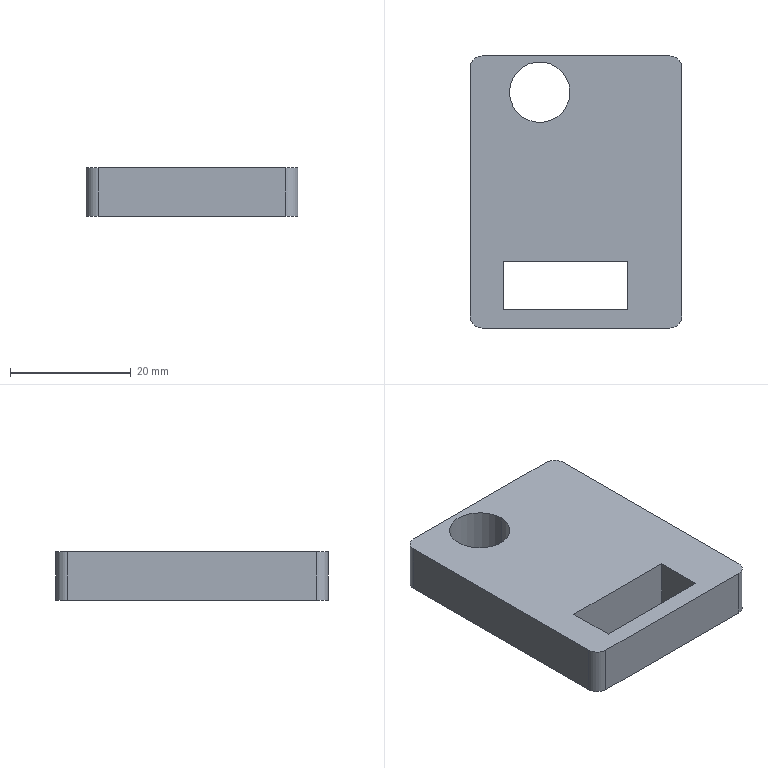Part | SolidWorks | features Fillet 1, FlatPattern 1, SMBaseFlange 1, SheetMetal 1 | 1 solid | 16 faces | box 35 x 45 x 8 mm | volume 10632 mm3 | plane 10 | cylinder 6 | commonest cylinder face diameters 4 x4 10 x2
STEP:
#1=CARTESIAN_POINT('',(-109.081,0.,8.));
#2=VERTEX_POINT('',#1);
#3=CARTESIAN_POINT('',(-99.081,0.,8.));
#4=VERTEX_POINT('',#3);
#5=CARTESIAN_POINT('',(-104.081,0.,8.));
#6=DIRECTION('',(0.,0.,1.));
#7=DIRECTION('',(1.,0.,0.));
#8=AXIS2_PLACEMENT_3D('',#5,#6,#7);
#9=CIRCLE('',#8,5.);
#10=EDGE_CURVE('',#2,#4,#9,.T.);
#11=ORIENTED_EDGE('',*,*,#10,.T.);
#12=CARTESIAN_POINT('',(-99.081,0.,0.));
#13=VERTEX_POINT('',#12);
#14=CARTESIAN_POINT('',(-99.081,0.,8.));
#15=DIRECTION('',(0.,0.,-1.));
#16=VECTOR('',#15,1000.);
#17=LINE('',#14,#16);
#18=EDGE_CURVE('',#4,#13,#17,.T.);
#19=ORIENTED_EDGE('',*,*,#18,.T.);
#20=CARTESIAN_POINT('',(-109.081,0.,0.));
#21=VERTEX_POINT('',#20);
#22=CARTESIAN_POINT('',(-104.081,0.,0.));
#23=DIRECTION('',(0.,0.,1.));
#24=DIRECTION('',(1.,0.,0.));
#25=AXIS2_PLACEMENT_3D('',#22,#23,#24);
#26=CIRCLE('',#25,5.);
#27=EDGE_CURVE('',#21,#13,#26,.T.);
#28=ORIENTED_EDGE('',*,*,#27,.F.);
#29=CARTESIAN_POINT('',(-109.081,0.,8.));
#30=DIRECTION('',(0.,0.,-1.));
#31=VECTOR('',#30,1000.);
#32=LINE('',#29,#31);
#33=EDGE_CURVE('',#2,#21,#32,.T.);
#34=ORIENTED_EDGE('',*,*,#33,.F.);
#35=EDGE_LOOP('',(#11,#19,#28,#34));
#36=FACE_OUTER_BOUND('',#35,.T.);
#37=CARTESIAN_POINT('',(-104.081,0.,8.));
#38=DIRECTION('',(0.,0.,-1.));
#39=DIRECTION('',(-1.,0.,0.));
#40=AXIS2_PLACEMENT_3D('',#37,#38,#39);
#41=CYLINDRICAL_SURFACE('',#40,5.);
#42=ADVANCED_FACE('',(#36),#41,.F.);
#43=ORIENTED_EDGE('',*,*,#10,.F.);
#44=CARTESIAN_POINT('',(-104.081,0.,8.));
#45=DIRECTION('',(0.,0.,1.));
#46=DIRECTION('',(1.,0.,0.));
#47=AXIS2_PLACEMENT_3D('',#44,#45,#46);
#48=CIRCLE('',#47,5.);
#49=EDGE_CURVE('',#4,#2,#48,.T.);
#50=ORIENTED_EDGE('',*,*,#49,.F.);
#51=EDGE_LOOP('',(#43,#50));
#52=FACE_BOUND('',#51,.T.);
#53=CARTESIAN_POINT('',(-115.581,4.,8.));
#54=VERTEX_POINT('',#53);
#55=CARTESIAN_POINT('',(-115.581,-37.,8.));
#56=VERTEX_POINT('',#55);
#57=CARTESIAN_POINT('',(-115.581,-39.,8.));
#58=DIRECTION('',(0.,-1.,0.));
#59=VECTOR('',#58,1000.);
#60=LINE('',#57,#59);
#61=EDGE_CURVE('',#54,#56,#60,.T.);
#62=ORIENTED_EDGE('',*,*,#61,.T.);
#63=CARTESIAN_POINT('',(-113.581,-39.,8.));
#64=VERTEX_POINT('',#63);
#65=CARTESIAN_POINT('',(-113.581,-37.,8.));
#66=DIRECTION('',(0.,0.,1.));
#67=DIRECTION('',(-1.,0.,0.));
#68=AXIS2_PLACEMENT_3D('',#65,#66,#67);
#69=CIRCLE('',#68,2.);
#70=EDGE_CURVE('',#56,#64,#69,.T.);
#71=ORIENTED_EDGE('',*,*,#70,.T.);
#72=CARTESIAN_POINT('',(-82.581,-39.,8.));
#73=VERTEX_POINT('',#72);
#74=CARTESIAN_POINT('',(-80.581,-39.,8.));
#75=DIRECTION('',(1.,0.,0.));
#76=VECTOR('',#75,1000.);
#77=LINE('',#74,#76);
#78=EDGE_CURVE('',#64,#73,#77,.T.);
#79=ORIENTED_EDGE('',*,*,#78,.T.);
#80=CARTESIAN_POINT('',(-80.581,-37.,8.));
#81=VERTEX_POINT('',#80);
#82=CARTESIAN_POINT('',(-82.581,-37.,8.));
#83=DIRECTION('',(0.,0.,1.));
#84=DIRECTION('',(-1.,0.,0.));
#85=AXIS2_PLACEMENT_3D('',#82,#83,#84);
#86=CIRCLE('',#85,2.);
#87=EDGE_CURVE('',#73,#81,#86,.T.);
#88=ORIENTED_EDGE('',*,*,#87,.T.);
#89=CARTESIAN_POINT('',(-80.581,4.,8.));
#90=VERTEX_POINT('',#89);
#91=CARTESIAN_POINT('',(-80.581,6.,8.));
#92=DIRECTION('',(0.,1.,0.));
#93=VECTOR('',#92,1000.);
#94=LINE('',#91,#93);
#95=EDGE_CURVE('',#81,#90,#94,.T.);
#96=ORIENTED_EDGE('',*,*,#95,.T.);
#97=CARTESIAN_POINT('',(-82.581,6.,8.));
#98=VERTEX_POINT('',#97);
#99=CARTESIAN_POINT('',(-82.581,4.,8.));
#100=DIRECTION('',(0.,0.,1.));
#101=DIRECTION('',(-1.,0.,0.));
#102=AXIS2_PLACEMENT_3D('',#99,#100,#101);
#103=CIRCLE('',#102,2.);
#104=EDGE_CURVE('',#90,#98,#103,.T.);
#105=ORIENTED_EDGE('',*,*,#104,.T.);
#106=CARTESIAN_POINT('',(-113.581,6.,8.));
#107=VERTEX_POINT('',#106);
#108=CARTESIAN_POINT('',(-115.581,6.,8.));
#109=DIRECTION('',(-1.,0.,0.));
#110=VECTOR('',#109,1000.);
#111=LINE('',#108,#110);
#112=EDGE_CURVE('',#98,#107,#111,.T.);
#113=ORIENTED_EDGE('',*,*,#112,.T.);
#114=CARTESIAN_POINT('',(-113.581,4.,8.));
#115=DIRECTION('',(0.,0.,1.));
#116=DIRECTION('',(-1.,0.,0.));
#117=AXIS2_PLACEMENT_3D('',#114,#115,#116);
#118=CIRCLE('',#117,2.);
#119=EDGE_CURVE('',#107,#54,#118,.T.);
#120=ORIENTED_EDGE('',*,*,#119,.T.);
#121=EDGE_LOOP('',(#62,#71,#79,#88,#96,#105,#113,#120));
#122=FACE_OUTER_BOUND('',#121,.T.);
#123=CARTESIAN_POINT('',(-110.081,-28.,8.));
#124=VERTEX_POINT('',#123);
#125=CARTESIAN_POINT('',(-110.081,-36.,8.));
#126=VERTEX_POINT('',#125);
#127=CARTESIAN_POINT('',(-110.081,-36.,8.));
#128=DIRECTION('',(0.,-1.,0.));
#129=VECTOR('',#128,1000.);
#130=LINE('',#127,#129);
#131=EDGE_CURVE('',#124,#126,#130,.T.);
#132=ORIENTED_EDGE('',*,*,#131,.F.);
#133=CARTESIAN_POINT('',(-89.581,-28.,8.));
#134=VERTEX_POINT('',#133);
#135=CARTESIAN_POINT('',(-110.081,-28.,8.));
#136=DIRECTION('',(-1.,0.,0.));
#137=VECTOR('',#136,1000.);
#138=LINE('',#135,#137);
#139=EDGE_CURVE('',#134,#124,#138,.T.);
#140=ORIENTED_EDGE('',*,*,#139,.F.);
#141=CARTESIAN_POINT('',(-89.581,-36.,8.));
#142=VERTEX_POINT('',#141);
#143=CARTESIAN_POINT('',(-89.581,-28.,8.));
#144=DIRECTION('',(0.,1.,0.));
#145=VECTOR('',#144,1000.);
#146=LINE('',#143,#145);
#147=EDGE_CURVE('',#142,#134,#146,.T.);
#148=ORIENTED_EDGE('',*,*,#147,.F.);
#149=CARTESIAN_POINT('',(-89.581,-36.,8.));
#150=DIRECTION('',(1.,0.,0.));
#151=VECTOR('',#150,1000.);
#152=LINE('',#149,#151);
#153=EDGE_CURVE('',#126,#142,#152,.T.);
#154=ORIENTED_EDGE('',*,*,#153,.F.);
#155=EDGE_LOOP('',(#132,#140,#148,#154));
#156=FACE_BOUND('',#155,.T.);
#157=CARTESIAN_POINT('',(0.,0.,8.));
#158=DIRECTION('',(0.,0.,-1.));
#159=DIRECTION('',(-1.,0.,0.));
#160=AXIS2_PLACEMENT_3D('',#157,#158,#159);
#161=PLANE('',#160);
#162=ADVANCED_FACE('',(#52,#122,#156),#161,.F.);
#163=CARTESIAN_POINT('',(-113.581,-39.,0.));
#164=VERTEX_POINT('',#163);
#165=CARTESIAN_POINT('',(-82.581,-39.,0.));
#166=VERTEX_POINT('',#165);
#167=CARTESIAN_POINT('',(-80.581,-39.,0.));
#168=DIRECTION('',(1.,0.,0.));
#169=VECTOR('',#168,1000.);
#170=LINE('',#167,#169);
#171=EDGE_CURVE('',#164,#166,#170,.T.);
#172=ORIENTED_EDGE('',*,*,#171,.F.);
#173=CARTESIAN_POINT('',(-115.581,-37.,0.));
#174=VERTEX_POINT('',#173);
#175=CARTESIAN_POINT('',(-113.581,-37.,0.));
#176=DIRECTION('',(0.,0.,-1.));
#177=DIRECTION('',(-1.,0.,0.));
#178=AXIS2_PLACEMENT_3D('',#175,#176,#177);
#179=CIRCLE('',#178,2.);
#180=EDGE_CURVE('',#164,#174,#179,.T.);
#181=ORIENTED_EDGE('',*,*,#180,.T.);
#182=CARTESIAN_POINT('',(-115.581,4.,0.));
#183=VERTEX_POINT('',#182);
#184=CARTESIAN_POINT('',(-115.581,-39.,0.));
#185=DIRECTION('',(0.,-1.,0.));
#186=VECTOR('',#185,1000.);
#187=LINE('',#184,#186);
#188=EDGE_CURVE('',#183,#174,#187,.T.);
#189=ORIENTED_EDGE('',*,*,#188,.F.);
#190=CARTESIAN_POINT('',(-113.581,6.,0.));
#191=VERTEX_POINT('',#190);
#192=CARTESIAN_POINT('',(-113.581,4.,0.));
#193=DIRECTION('',(0.,0.,-1.));
#194=DIRECTION('',(-1.,0.,0.));
#195=AXIS2_PLACEMENT_3D('',#192,#193,#194);
#196=CIRCLE('',#195,2.);
#197=EDGE_CURVE('',#183,#191,#196,.T.);
#198=ORIENTED_EDGE('',*,*,#197,.T.);
#199=CARTESIAN_POINT('',(-82.581,6.,0.));
#200=VERTEX_POINT('',#199);
#201=CARTESIAN_POINT('',(-115.581,6.,0.));
#202=DIRECTION('',(-1.,0.,0.));
#203=VECTOR('',#202,1000.);
#204=LINE('',#201,#203);
#205=EDGE_CURVE('',#200,#191,#204,.T.);
#206=ORIENTED_EDGE('',*,*,#205,.F.);
#207=CARTESIAN_POINT('',(-80.581,4.,0.));
#208=VERTEX_POINT('',#207);
#209=CARTESIAN_POINT('',(-82.581,4.,0.));
#210=DIRECTION('',(0.,0.,-1.));
#211=DIRECTION('',(-1.,0.,0.));
#212=AXIS2_PLACEMENT_3D('',#209,#210,#211);
#213=CIRCLE('',#212,2.);
#214=EDGE_CURVE('',#200,#208,#213,.T.);
#215=ORIENTED_EDGE('',*,*,#214,.T.);
#216=CARTESIAN_POINT('',(-80.581,-37.,0.));
#217=VERTEX_POINT('',#216);
#218=CARTESIAN_POINT('',(-80.581,6.,0.));
#219=DIRECTION('',(0.,1.,0.));
#220=VECTOR('',#219,1000.);
#221=LINE('',#218,#220);
#222=EDGE_CURVE('',#217,#208,#221,.T.);
#223=ORIENTED_EDGE('',*,*,#222,.F.);
#224=CARTESIAN_POINT('',(-82.581,-37.,0.));
#225=DIRECTION('',(0.,0.,-1.));
#226=DIRECTION('',(-1.,0.,0.));
#227=AXIS2_PLACEMENT_3D('',#224,#225,#226);
#228=CIRCLE('',#227,2.);
#229=EDGE_CURVE('',#217,#166,#228,.T.);
#230=ORIENTED_EDGE('',*,*,#229,.T.);
#231=EDGE_LOOP('',(#172,#181,#189,#198,#206,#215,#223,#230));
#232=FACE_OUTER_BOUND('',#231,.T.);
#233=ORIENTED_EDGE('',*,*,#27,.T.);
#234=CARTESIAN_POINT('',(-104.081,0.,0.));
#235=DIRECTION('',(0.,0.,1.));
#236=DIRECTION('',(1.,0.,0.));
#237=AXIS2_PLACEMENT_3D('',#234,#235,#236);
#238=CIRCLE('',#237,5.);
#239=EDGE_CURVE('',#13,#21,#238,.T.);
#240=ORIENTED_EDGE('',*,*,#239,.T.);
#241=EDGE_LOOP('',(#233,#240));
#242=FACE_BOUND('',#241,.T.);
#243=CARTESIAN_POINT('',(-89.581,-28.,0.));
#244=VERTEX_POINT('',#243);
#245=CARTESIAN_POINT('',(-110.081,-28.,0.));
#246=VERTEX_POINT('',#245);
#247=CARTESIAN_POINT('',(-110.081,-28.,0.));
#248=DIRECTION('',(-1.,0.,0.));
#249=VECTOR('',#248,1000.);
#250=LINE('',#247,#249);
#251=EDGE_CURVE('',#244,#246,#250,.T.);
#252=ORIENTED_EDGE('',*,*,#251,.T.);
#253=CARTESIAN_POINT('',(-110.081,-36.,0.));
#254=VERTEX_POINT('',#253);
#255=CARTESIAN_POINT('',(-110.081,-36.,0.));
#256=DIRECTION('',(0.,-1.,0.));
#257=VECTOR('',#256,1000.);
#258=LINE('',#255,#257);
#259=EDGE_CURVE('',#246,#254,#258,.T.);
#260=ORIENTED_EDGE('',*,*,#259,.T.);
#261=CARTESIAN_POINT('',(-89.581,-36.,0.));
#262=VERTEX_POINT('',#261);
#263=CARTESIAN_POINT('',(-89.581,-36.,0.));
#264=DIRECTION('',(1.,0.,0.));
#265=VECTOR('',#264,1000.);
#266=LINE('',#263,#265);
#267=EDGE_CURVE('',#254,#262,#266,.T.);
#268=ORIENTED_EDGE('',*,*,#267,.T.);
#269=CARTESIAN_POINT('',(-89.581,-28.,0.));
#270=DIRECTION('',(0.,1.,0.));
#271=VECTOR('',#270,1000.);
#272=LINE('',#269,#271);
#273=EDGE_CURVE('',#262,#244,#272,.T.);
#274=ORIENTED_EDGE('',*,*,#273,.T.);
#275=EDGE_LOOP('',(#252,#260,#268,#274));
#276=FACE_BOUND('',#275,.T.);
#277=CARTESIAN_POINT('',(0.,0.,0.));
#278=DIRECTION('',(0.,0.,-1.));
#279=DIRECTION('',(-1.,0.,0.));
#280=AXIS2_PLACEMENT_3D('',#277,#278,#279);
#281=PLANE('',#280);
#282=ADVANCED_FACE('',(#232,#242,#276),#281,.T.);
#283=ORIENTED_EDGE('',*,*,#188,.T.);
#284=CARTESIAN_POINT('',(-115.581,-37.,8.));
#285=DIRECTION('',(0.,0.,1.));
#286=VECTOR('',#285,1000.);
#287=LINE('',#284,#286);
#288=EDGE_CURVE('',#174,#56,#287,.T.);
#289=ORIENTED_EDGE('',*,*,#288,.T.);
#290=ORIENTED_EDGE('',*,*,#61,.F.);
#291=CARTESIAN_POINT('',(-115.581,4.,8.));
#292=DIRECTION('',(0.,0.,-1.));
#293=VECTOR('',#292,1000.);
#294=LINE('',#291,#293);
#295=EDGE_CURVE('',#54,#183,#294,.T.);
#296=ORIENTED_EDGE('',*,*,#295,.T.);
#297=EDGE_LOOP('',(#283,#289,#290,#296));
#298=FACE_OUTER_BOUND('',#297,.T.);
#299=CARTESIAN_POINT('',(-115.581,-39.,8.));
#300=DIRECTION('',(1.,0.,0.));
#301=DIRECTION('',(0.,0.,-1.));
#302=AXIS2_PLACEMENT_3D('',#299,#300,#301);
#303=PLANE('',#302);
#304=ADVANCED_FACE('',(#298),#303,.F.);
#305=ORIENTED_EDGE('',*,*,#78,.F.);
#306=CARTESIAN_POINT('',(-113.581,-39.,8.));
#307=DIRECTION('',(0.,0.,-1.));
#308=VECTOR('',#307,1000.);
#309=LINE('',#306,#308);
#310=EDGE_CURVE('',#64,#164,#309,.T.);
#311=ORIENTED_EDGE('',*,*,#310,.T.);
#312=ORIENTED_EDGE('',*,*,#171,.T.);
#313=CARTESIAN_POINT('',(-82.581,-39.,8.));
#314=DIRECTION('',(0.,0.,1.));
#315=VECTOR('',#314,1000.);
#316=LINE('',#313,#315);
#317=EDGE_CURVE('',#166,#73,#316,.T.);
#318=ORIENTED_EDGE('',*,*,#317,.T.);
#319=EDGE_LOOP('',(#305,#311,#312,#318));
#320=FACE_OUTER_BOUND('',#319,.T.);
#321=CARTESIAN_POINT('',(-80.581,-39.,8.));
#322=DIRECTION('',(0.,1.,0.));
#323=DIRECTION('',(-1.,0.,0.));
#324=AXIS2_PLACEMENT_3D('',#321,#322,#323);
#325=PLANE('',#324);
#326=ADVANCED_FACE('',(#320),#325,.F.);
#327=ORIENTED_EDGE('',*,*,#95,.F.);
#328=CARTESIAN_POINT('',(-80.581,-37.,8.));
#329=DIRECTION('',(0.,0.,-1.));
#330=VECTOR('',#329,1000.);
#331=LINE('',#328,#330);
#332=EDGE_CURVE('',#81,#217,#331,.T.);
#333=ORIENTED_EDGE('',*,*,#332,.T.);
#334=ORIENTED_EDGE('',*,*,#222,.T.);
#335=CARTESIAN_POINT('',(-80.581,4.,8.));
#336=DIRECTION('',(0.,0.,1.));
#337=VECTOR('',#336,1000.);
#338=LINE('',#335,#337);
#339=EDGE_CURVE('',#208,#90,#338,.T.);
#340=ORIENTED_EDGE('',*,*,#339,.T.);
#341=EDGE_LOOP('',(#327,#333,#334,#340));
#342=FACE_OUTER_BOUND('',#341,.T.);
#343=CARTESIAN_POINT('',(-80.581,6.,8.));
#344=DIRECTION('',(-1.,0.,0.));
#345=DIRECTION('',(0.,0.,1.));
#346=AXIS2_PLACEMENT_3D('',#343,#344,#345);
#347=PLANE('',#346);
#348=ADVANCED_FACE('',(#342),#347,.F.);
#349=ORIENTED_EDGE('',*,*,#112,.F.);
#350=CARTESIAN_POINT('',(-82.581,6.,8.));
#351=DIRECTION('',(0.,0.,-1.));
#352=VECTOR('',#351,1000.);
#353=LINE('',#350,#352);
#354=EDGE_CURVE('',#98,#200,#353,.T.);
#355=ORIENTED_EDGE('',*,*,#354,.T.);
#356=ORIENTED_EDGE('',*,*,#205,.T.);
#357=CARTESIAN_POINT('',(-113.581,6.,8.));
#358=DIRECTION('',(0.,0.,1.));
#359=VECTOR('',#358,1000.);
#360=LINE('',#357,#359);
#361=EDGE_CURVE('',#191,#107,#360,.T.);
#362=ORIENTED_EDGE('',*,*,#361,.T.);
#363=EDGE_LOOP('',(#349,#355,#356,#362));
#364=FACE_OUTER_BOUND('',#363,.T.);
#365=CARTESIAN_POINT('',(-115.581,6.,8.));
#366=DIRECTION('',(0.,-1.,0.));
#367=DIRECTION('',(0.,0.,-1.));
#368=AXIS2_PLACEMENT_3D('',#365,#366,#367);
#369=PLANE('',#368);
#370=ADVANCED_FACE('',(#364),#369,.F.);
#371=ORIENTED_EDGE('',*,*,#18,.F.);
#372=ORIENTED_EDGE('',*,*,#49,.T.);
#373=ORIENTED_EDGE('',*,*,#33,.T.);
#374=ORIENTED_EDGE('',*,*,#239,.F.);
#375=EDGE_LOOP('',(#371,#372,#373,#374));
#376=FACE_OUTER_BOUND('',#375,.T.);
#377=CARTESIAN_POINT('',(-104.081,0.,8.));
#378=DIRECTION('',(0.,0.,-1.));
#379=DIRECTION('',(-1.,0.,0.));
#380=AXIS2_PLACEMENT_3D('',#377,#378,#379);
#381=CYLINDRICAL_SURFACE('',#380,5.);
#382=ADVANCED_FACE('',(#376),#381,.F.);
#383=ORIENTED_EDGE('',*,*,#259,.F.);
#384=CARTESIAN_POINT('',(-110.081,-28.,8.));
#385=DIRECTION('',(0.,0.,-1.));
#386=VECTOR('',#385,1000.);
#387=LINE('',#384,#386);
#388=EDGE_CURVE('',#124,#246,#387,.T.);
#389=ORIENTED_EDGE('',*,*,#388,.F.);
#390=ORIENTED_EDGE('',*,*,#131,.T.);
#391=CARTESIAN_POINT('',(-110.081,-36.,8.));
#392=DIRECTION('',(0.,0.,-1.));
#393=VECTOR('',#392,1000.);
#394=LINE('',#391,#393);
#395=EDGE_CURVE('',#126,#254,#394,.T.);
#396=ORIENTED_EDGE('',*,*,#395,.T.);
#397=EDGE_LOOP('',(#383,#389,#390,#396));
#398=FACE_OUTER_BOUND('',#397,.T.);
#399=CARTESIAN_POINT('',(-110.081,-36.,8.));
#400=DIRECTION('',(1.,0.,0.));
#401=DIRECTION('',(0.,0.,-1.));
#402=AXIS2_PLACEMENT_3D('',#399,#400,#401);
#403=PLANE('',#402);
#404=ADVANCED_FACE('',(#398),#403,.T.);
#405=ORIENTED_EDGE('',*,*,#267,.F.);
#406=ORIENTED_EDGE('',*,*,#395,.F.);
#407=ORIENTED_EDGE('',*,*,#153,.T.);
#408=CARTESIAN_POINT('',(-89.581,-36.,8.));
#409=DIRECTION('',(0.,0.,-1.));
#410=VECTOR('',#409,1000.);
#411=LINE('',#408,#410);
#412=EDGE_CURVE('',#142,#262,#411,.T.);
#413=ORIENTED_EDGE('',*,*,#412,.T.);
#414=EDGE_LOOP('',(#405,#406,#407,#413));
#415=FACE_OUTER_BOUND('',#414,.T.);
#416=CARTESIAN_POINT('',(-89.581,-36.,8.));
#417=DIRECTION('',(0.,1.,0.));
#418=DIRECTION('',(0.,0.,1.));
#419=AXIS2_PLACEMENT_3D('',#416,#417,#418);
#420=PLANE('',#419);
#421=ADVANCED_FACE('',(#415),#420,.T.);
#422=ORIENTED_EDGE('',*,*,#273,.F.);
#423=ORIENTED_EDGE('',*,*,#412,.F.);
#424=ORIENTED_EDGE('',*,*,#147,.T.);
#425=CARTESIAN_POINT('',(-89.581,-28.,8.));
#426=DIRECTION('',(0.,0.,-1.));
#427=VECTOR('',#426,1000.);
#428=LINE('',#425,#427);
#429=EDGE_CURVE('',#134,#244,#428,.T.);
#430=ORIENTED_EDGE('',*,*,#429,.T.);
#431=EDGE_LOOP('',(#422,#423,#424,#430));
#432=FACE_OUTER_BOUND('',#431,.T.);
#433=CARTESIAN_POINT('',(-89.581,-28.,8.));
#434=DIRECTION('',(-1.,0.,0.));
#435=DIRECTION('',(0.,0.,1.));
#436=AXIS2_PLACEMENT_3D('',#433,#434,#435);
#437=PLANE('',#436);
#438=ADVANCED_FACE('',(#432),#437,.T.);
#439=ORIENTED_EDGE('',*,*,#251,.F.);
#440=ORIENTED_EDGE('',*,*,#429,.F.);
#441=ORIENTED_EDGE('',*,*,#139,.T.);
#442=ORIENTED_EDGE('',*,*,#388,.T.);
#443=EDGE_LOOP('',(#439,#440,#441,#442));
#444=FACE_OUTER_BOUND('',#443,.T.);
#445=CARTESIAN_POINT('',(-110.081,-28.,8.));
#446=DIRECTION('',(0.,-1.,0.));
#447=DIRECTION('',(0.,0.,-1.));
#448=AXIS2_PLACEMENT_3D('',#445,#446,#447);
#449=PLANE('',#448);
#450=ADVANCED_FACE('',(#444),#449,.T.);
#451=ORIENTED_EDGE('',*,*,#70,.F.);
#452=ORIENTED_EDGE('',*,*,#288,.F.);
#453=ORIENTED_EDGE('',*,*,#180,.F.);
#454=ORIENTED_EDGE('',*,*,#310,.F.);
#455=EDGE_LOOP('',(#451,#452,#453,#454));
#456=FACE_OUTER_BOUND('',#455,.T.);
#457=CARTESIAN_POINT('',(-113.581,-37.,8.));
#458=DIRECTION('',(0.,0.,-1.));
#459=DIRECTION('',(-1.,0.,0.));
#460=AXIS2_PLACEMENT_3D('',#457,#458,#459);
#461=CYLINDRICAL_SURFACE('',#460,2.);
#462=ADVANCED_FACE('',(#456),#461,.T.);
#463=ORIENTED_EDGE('',*,*,#87,.F.);
#464=ORIENTED_EDGE('',*,*,#317,.F.);
#465=ORIENTED_EDGE('',*,*,#229,.F.);
#466=ORIENTED_EDGE('',*,*,#332,.F.);
#467=EDGE_LOOP('',(#463,#464,#465,#466));
#468=FACE_OUTER_BOUND('',#467,.T.);
#469=CARTESIAN_POINT('',(-82.581,-37.,8.));
#470=DIRECTION('',(0.,0.,-1.));
#471=DIRECTION('',(-1.,0.,0.));
#472=AXIS2_PLACEMENT_3D('',#469,#470,#471);
#473=CYLINDRICAL_SURFACE('',#472,2.);
#474=ADVANCED_FACE('',(#468),#473,.T.);
#475=ORIENTED_EDGE('',*,*,#104,.F.);
#476=ORIENTED_EDGE('',*,*,#339,.F.);
#477=ORIENTED_EDGE('',*,*,#214,.F.);
#478=ORIENTED_EDGE('',*,*,#354,.F.);
#479=EDGE_LOOP('',(#475,#476,#477,#478));
#480=FACE_OUTER_BOUND('',#479,.T.);
#481=CARTESIAN_POINT('',(-82.581,4.,8.));
#482=DIRECTION('',(0.,0.,-1.));
#483=DIRECTION('',(-1.,0.,0.));
#484=AXIS2_PLACEMENT_3D('',#481,#482,#483);
#485=CYLINDRICAL_SURFACE('',#484,2.);
#486=ADVANCED_FACE('',(#480),#485,.T.);
#487=ORIENTED_EDGE('',*,*,#119,.F.);
#488=ORIENTED_EDGE('',*,*,#361,.F.);
#489=ORIENTED_EDGE('',*,*,#197,.F.);
#490=ORIENTED_EDGE('',*,*,#295,.F.);
#491=EDGE_LOOP('',(#487,#488,#489,#490));
#492=FACE_OUTER_BOUND('',#491,.T.);
#493=CARTESIAN_POINT('',(-113.581,4.,8.));
#494=DIRECTION('',(0.,0.,-1.));
#495=DIRECTION('',(-1.,0.,0.));
#496=AXIS2_PLACEMENT_3D('',#493,#494,#495);
#497=CYLINDRICAL_SURFACE('',#496,2.);
#498=ADVANCED_FACE('',(#492),#497,.T.);
#499=CLOSED_SHELL('',(#42,#162,#282,#304,#326,#348,#370,#382,#404,#421,#438,#450,#462,#474,#486,#498));
#500=MANIFOLD_SOLID_BREP('',#499);
#501=CARTESIAN_POINT('',(0.,0.,0.));
#502=DIRECTION('',(0.,0.,1.));
#503=DIRECTION('',(1.,0.,0.));
#504=AXIS2_PLACEMENT_3D('',#501,#502,#503);
#505=(LENGTH_UNIT()NAMED_UNIT(*)SI_UNIT(.MILLI.,.METRE.));
#506=UNCERTAINTY_MEASURE_WITH_UNIT(LENGTH_MEASURE(0.00001),#505,'','');
#507=(NAMED_UNIT(*)PLANE_ANGLE_UNIT()SI_UNIT($,.RADIAN.));
#508=(NAMED_UNIT(*)SI_UNIT($,.STERADIAN.)SOLID_ANGLE_UNIT());
#509=(GEOMETRIC_REPRESENTATION_CONTEXT(3)GLOBAL_UNCERTAINTY_ASSIGNED_CONTEXT((#506))GLOBAL_UNIT_ASSIGNED_CONTEXT((#505,#507,#508))REPRESENTATION_CONTEXT('',''));
#510=ADVANCED_BREP_SHAPE_REPRESENTATION('',(#500,#504),#509);